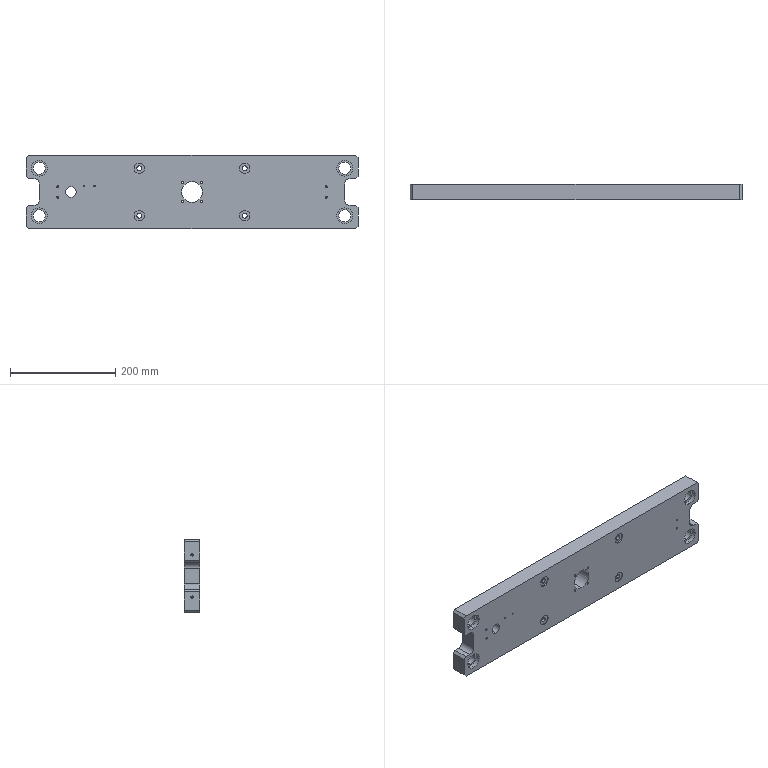Part | SolidWorks | features BaseBody 1 | 1 solid | 202 faces | box 630 x 30 x 140 mm | volume 2444108 mm3 | cylinder 112 | cone 56 | plane 34 | commonest cylinder face diameters 3.3 x24 5 x20 4.2 x16 20 x14 9 x8 15 x8